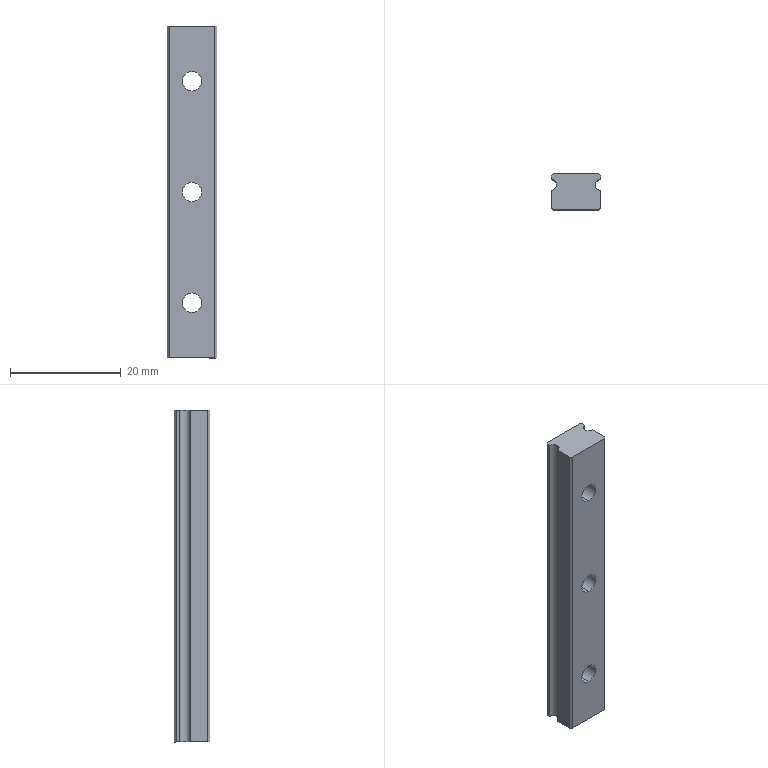Part | SolidWorks | features BaseBody 1, ICE 1 | 1 solid | 30 faces | box 9 x 6.5 x 60 mm | volume 2919 mm3 | cylinder 15 | plane 15 | commonest cylinder face diameters 3.5 x6 6 x6 2 x3
STEP:
#1=CARTESIAN_POINT('',(0.,0.,-55.85));
#2=VERTEX_POINT('',#1);
#3=CARTESIAN_POINT('',(0.,0.,-59.35));
#4=VERTEX_POINT('',#3);
#5=CARTESIAN_POINT('',(0.,0.,-57.6));
#6=DIRECTION('',(0.,-1.,0.));
#7=DIRECTION('',(0.,0.,1.));
#8=AXIS2_PLACEMENT_3D('',#5,#6,#7);
#9=CIRCLE('',#8,1.75);
#10=EDGE_CURVE('',#2,#4,#9,.T.);
#11=ORIENTED_EDGE('',*,*,#10,.T.);
#12=CARTESIAN_POINT('',(0.,3.,-59.35));
#13=VERTEX_POINT('',#12);
#14=CARTESIAN_POINT('',(0.,-94.114,-59.35));
#15=DIRECTION('',(0.,1.,0.));
#16=VECTOR('',#15,1000.);
#17=LINE('',#14,#16);
#18=EDGE_CURVE('',#4,#13,#17,.T.);
#19=ORIENTED_EDGE('',*,*,#18,.T.);
#20=CARTESIAN_POINT('',(0.,3.,-55.85));
#21=VERTEX_POINT('',#20);
#22=CARTESIAN_POINT('',(0.,3.,-57.6));
#23=DIRECTION('',(0.,-1.,0.));
#24=DIRECTION('',(0.,0.,1.));
#25=AXIS2_PLACEMENT_3D('',#22,#23,#24);
#26=CIRCLE('',#25,1.75);
#27=EDGE_CURVE('',#21,#13,#26,.T.);
#28=ORIENTED_EDGE('',*,*,#27,.F.);
#29=CARTESIAN_POINT('',(0.,-94.114,-55.85));
#30=DIRECTION('',(0.,1.,0.));
#31=VECTOR('',#30,1000.);
#32=LINE('',#29,#31);
#33=EDGE_CURVE('',#2,#21,#32,.T.);
#34=ORIENTED_EDGE('',*,*,#33,.F.);
#35=EDGE_LOOP('',(#11,#19,#28,#34));
#36=FACE_OUTER_BOUND('',#35,.T.);
#37=CARTESIAN_POINT('',(0.,-94.114,-57.6));
#38=DIRECTION('',(0.,1.,0.));
#39=DIRECTION('',(0.,0.,1.));
#40=AXIS2_PLACEMENT_3D('',#37,#38,#39);
#41=CYLINDRICAL_SURFACE('',#40,1.75);
#42=ADVANCED_FACE('',(#36),#41,.F.);
#43=CARTESIAN_POINT('',(0.,0.,-75.85));
#44=VERTEX_POINT('',#43);
#45=CARTESIAN_POINT('',(0.,0.,-79.35));
#46=VERTEX_POINT('',#45);
#47=CARTESIAN_POINT('',(0.,0.,-77.6));
#48=DIRECTION('',(0.,-1.,0.));
#49=DIRECTION('',(0.,0.,1.));
#50=AXIS2_PLACEMENT_3D('',#47,#48,#49);
#51=CIRCLE('',#50,1.75);
#52=EDGE_CURVE('',#44,#46,#51,.T.);
#53=ORIENTED_EDGE('',*,*,#52,.T.);
#54=CARTESIAN_POINT('',(0.,3.,-79.35));
#55=VERTEX_POINT('',#54);
#56=CARTESIAN_POINT('',(0.,-94.114,-79.35));
#57=DIRECTION('',(0.,1.,0.));
#58=VECTOR('',#57,1000.);
#59=LINE('',#56,#58);
#60=EDGE_CURVE('',#46,#55,#59,.T.);
#61=ORIENTED_EDGE('',*,*,#60,.T.);
#62=CARTESIAN_POINT('',(0.,3.,-75.85));
#63=VERTEX_POINT('',#62);
#64=CARTESIAN_POINT('',(0.,3.,-77.6));
#65=DIRECTION('',(0.,-1.,0.));
#66=DIRECTION('',(0.,0.,1.));
#67=AXIS2_PLACEMENT_3D('',#64,#65,#66);
#68=CIRCLE('',#67,1.75);
#69=EDGE_CURVE('',#63,#55,#68,.T.);
#70=ORIENTED_EDGE('',*,*,#69,.F.);
#71=CARTESIAN_POINT('',(0.,-94.114,-75.85));
#72=DIRECTION('',(0.,1.,0.));
#73=VECTOR('',#72,1000.);
#74=LINE('',#71,#73);
#75=EDGE_CURVE('',#44,#63,#74,.T.);
#76=ORIENTED_EDGE('',*,*,#75,.F.);
#77=EDGE_LOOP('',(#53,#61,#70,#76));
#78=FACE_OUTER_BOUND('',#77,.T.);
#79=CARTESIAN_POINT('',(0.,-94.114,-77.6));
#80=DIRECTION('',(0.,1.,0.));
#81=DIRECTION('',(0.,0.,1.));
#82=AXIS2_PLACEMENT_3D('',#79,#80,#81);
#83=CYLINDRICAL_SURFACE('',#82,1.75);
#84=ADVANCED_FACE('',(#78),#83,.F.);
#85=CARTESIAN_POINT('',(0.,0.,-95.85));
#86=VERTEX_POINT('',#85);
#87=CARTESIAN_POINT('',(0.,0.,-99.35));
#88=VERTEX_POINT('',#87);
#89=CARTESIAN_POINT('',(0.,0.,-97.6));
#90=DIRECTION('',(0.,-1.,0.));
#91=DIRECTION('',(0.,0.,1.));
#92=AXIS2_PLACEMENT_3D('',#89,#90,#91);
#93=CIRCLE('',#92,1.75);
#94=EDGE_CURVE('',#86,#88,#93,.T.);
#95=ORIENTED_EDGE('',*,*,#94,.T.);
#96=CARTESIAN_POINT('',(0.,3.,-99.35));
#97=VERTEX_POINT('',#96);
#98=CARTESIAN_POINT('',(0.,-94.114,-99.35));
#99=DIRECTION('',(0.,1.,0.));
#100=VECTOR('',#99,1000.);
#101=LINE('',#98,#100);
#102=EDGE_CURVE('',#88,#97,#101,.T.);
#103=ORIENTED_EDGE('',*,*,#102,.T.);
#104=CARTESIAN_POINT('',(0.,3.,-95.85));
#105=VERTEX_POINT('',#104);
#106=CARTESIAN_POINT('',(0.,3.,-97.6));
#107=DIRECTION('',(0.,-1.,0.));
#108=DIRECTION('',(0.,0.,1.));
#109=AXIS2_PLACEMENT_3D('',#106,#107,#108);
#110=CIRCLE('',#109,1.75);
#111=EDGE_CURVE('',#105,#97,#110,.T.);
#112=ORIENTED_EDGE('',*,*,#111,.F.);
#113=CARTESIAN_POINT('',(0.,-94.114,-95.85));
#114=DIRECTION('',(0.,1.,0.));
#115=VECTOR('',#114,1000.);
#116=LINE('',#113,#115);
#117=EDGE_CURVE('',#86,#105,#116,.T.);
#118=ORIENTED_EDGE('',*,*,#117,.F.);
#119=EDGE_LOOP('',(#95,#103,#112,#118));
#120=FACE_OUTER_BOUND('',#119,.T.);
#121=CARTESIAN_POINT('',(0.,-94.114,-97.6));
#122=DIRECTION('',(0.,1.,0.));
#123=DIRECTION('',(0.,0.,1.));
#124=AXIS2_PLACEMENT_3D('',#121,#122,#123);
#125=CYLINDRICAL_SURFACE('',#124,1.75);
#126=ADVANCED_FACE('',(#120),#125,.F.);
#127=CARTESIAN_POINT('',(4.5,5.5,-47.6));
#128=VERTEX_POINT('',#127);
#129=CARTESIAN_POINT('',(3.5,4.5,-47.6));
#130=VERTEX_POINT('',#129);
#131=CARTESIAN_POINT('',(4.5,4.5,-47.6));
#132=DIRECTION('',(0.,0.,1.));
#133=DIRECTION('',(-1.,0.,0.));
#134=AXIS2_PLACEMENT_3D('',#131,#132,#133);
#135=CIRCLE('',#134,1.);
#136=EDGE_CURVE('',#128,#130,#135,.T.);
#137=ORIENTED_EDGE('',*,*,#136,.T.);
#138=CARTESIAN_POINT('',(3.5,4.5,-107.6));
#139=VERTEX_POINT('',#138);
#140=CARTESIAN_POINT('',(3.5,4.5,27.5));
#141=DIRECTION('',(0.,0.,-1.));
#142=VECTOR('',#141,1000.);
#143=LINE('',#140,#142);
#144=EDGE_CURVE('',#130,#139,#143,.T.);
#145=ORIENTED_EDGE('',*,*,#144,.T.);
#146=CARTESIAN_POINT('',(4.5,5.5,-107.6));
#147=VERTEX_POINT('',#146);
#148=CARTESIAN_POINT('',(4.5,4.5,-107.6));
#149=DIRECTION('',(0.,0.,-1.));
#150=DIRECTION('',(-1.,0.,0.));
#151=AXIS2_PLACEMENT_3D('',#148,#149,#150);
#152=CIRCLE('',#151,1.);
#153=EDGE_CURVE('',#139,#147,#152,.T.);
#154=ORIENTED_EDGE('',*,*,#153,.T.);
#155=CARTESIAN_POINT('',(4.5,5.5,27.5));
#156=DIRECTION('',(0.,0.,-1.));
#157=VECTOR('',#156,1000.);
#158=LINE('',#155,#157);
#159=EDGE_CURVE('',#128,#147,#158,.T.);
#160=ORIENTED_EDGE('',*,*,#159,.F.);
#161=EDGE_LOOP('',(#137,#145,#154,#160));
#162=FACE_OUTER_BOUND('',#161,.T.);
#163=CARTESIAN_POINT('',(4.5,4.5,27.5));
#164=DIRECTION('',(0.,0.,-1.));
#165=DIRECTION('',(-1.,0.,0.));
#166=AXIS2_PLACEMENT_3D('',#163,#164,#165);
#167=CYLINDRICAL_SURFACE('',#166,1.);
#168=ADVANCED_FACE('',(#162),#167,.F.);
#169=CARTESIAN_POINT('',(0.,3.,-60.6));
#170=VERTEX_POINT('',#169);
#171=CARTESIAN_POINT('',(0.,3.,-54.6));
#172=VERTEX_POINT('',#171);
#173=CARTESIAN_POINT('',(0.,3.,-57.6));
#174=DIRECTION('',(0.,1.,0.));
#175=DIRECTION('',(0.,0.,1.));
#176=AXIS2_PLACEMENT_3D('',#173,#174,#175);
#177=CIRCLE('',#176,3.);
#178=EDGE_CURVE('',#170,#172,#177,.T.);
#179=ORIENTED_EDGE('',*,*,#178,.F.);
#180=CARTESIAN_POINT('',(0.,6.5,-60.6));
#181=VERTEX_POINT('',#180);
#182=CARTESIAN_POINT('',(0.,4.75,-60.6));
#183=DIRECTION('',(0.,1.,0.));
#184=VECTOR('',#183,1000.);
#185=LINE('',#182,#184);
#186=EDGE_CURVE('',#170,#181,#185,.T.);
#187=ORIENTED_EDGE('',*,*,#186,.T.);
#188=CARTESIAN_POINT('',(0.,6.5,-54.6));
#189=VERTEX_POINT('',#188);
#190=CARTESIAN_POINT('',(0.,6.5,-57.6));
#191=DIRECTION('',(0.,1.,0.));
#192=DIRECTION('',(0.,0.,1.));
#193=AXIS2_PLACEMENT_3D('',#190,#191,#192);
#194=CIRCLE('',#193,3.);
#195=EDGE_CURVE('',#181,#189,#194,.T.);
#196=ORIENTED_EDGE('',*,*,#195,.T.);
#197=CARTESIAN_POINT('',(0.,4.75,-54.6));
#198=DIRECTION('',(0.,1.,0.));
#199=VECTOR('',#198,1000.);
#200=LINE('',#197,#199);
#201=EDGE_CURVE('',#172,#189,#200,.T.);
#202=ORIENTED_EDGE('',*,*,#201,.F.);
#203=EDGE_LOOP('',(#179,#187,#196,#202));
#204=FACE_OUTER_BOUND('',#203,.T.);
#205=CARTESIAN_POINT('',(0.,4.75,-57.6));
#206=DIRECTION('',(0.,1.,0.));
#207=DIRECTION('',(0.,0.,1.));
#208=AXIS2_PLACEMENT_3D('',#205,#206,#207);
#209=CYLINDRICAL_SURFACE('',#208,3.);
#210=ADVANCED_FACE('',(#204),#209,.F.);
#211=CARTESIAN_POINT('',(0.,3.,-80.6));
#212=VERTEX_POINT('',#211);
#213=CARTESIAN_POINT('',(0.,3.,-74.6));
#214=VERTEX_POINT('',#213);
#215=CARTESIAN_POINT('',(0.,3.,-77.6));
#216=DIRECTION('',(0.,1.,0.));
#217=DIRECTION('',(0.,0.,1.));
#218=AXIS2_PLACEMENT_3D('',#215,#216,#217);
#219=CIRCLE('',#218,3.);
#220=EDGE_CURVE('',#212,#214,#219,.T.);
#221=ORIENTED_EDGE('',*,*,#220,.F.);
#222=CARTESIAN_POINT('',(0.,6.5,-80.6));
#223=VERTEX_POINT('',#222);
#224=CARTESIAN_POINT('',(0.,4.75,-80.6));
#225=DIRECTION('',(0.,1.,0.));
#226=VECTOR('',#225,1000.);
#227=LINE('',#224,#226);
#228=EDGE_CURVE('',#212,#223,#227,.T.);
#229=ORIENTED_EDGE('',*,*,#228,.T.);
#230=CARTESIAN_POINT('',(0.,6.5,-74.6));
#231=VERTEX_POINT('',#230);
#232=CARTESIAN_POINT('',(0.,6.5,-77.6));
#233=DIRECTION('',(0.,1.,0.));
#234=DIRECTION('',(0.,0.,1.));
#235=AXIS2_PLACEMENT_3D('',#232,#233,#234);
#236=CIRCLE('',#235,3.);
#237=EDGE_CURVE('',#223,#231,#236,.T.);
#238=ORIENTED_EDGE('',*,*,#237,.T.);
#239=CARTESIAN_POINT('',(0.,4.75,-74.6));
#240=DIRECTION('',(0.,1.,0.));
#241=VECTOR('',#240,1000.);
#242=LINE('',#239,#241);
#243=EDGE_CURVE('',#214,#231,#242,.T.);
#244=ORIENTED_EDGE('',*,*,#243,.F.);
#245=EDGE_LOOP('',(#221,#229,#238,#244));
#246=FACE_OUTER_BOUND('',#245,.T.);
#247=CARTESIAN_POINT('',(0.,4.75,-77.6));
#248=DIRECTION('',(0.,1.,0.));
#249=DIRECTION('',(0.,0.,1.));
#250=AXIS2_PLACEMENT_3D('',#247,#248,#249);
#251=CYLINDRICAL_SURFACE('',#250,3.);
#252=ADVANCED_FACE('',(#246),#251,.F.);
#253=CARTESIAN_POINT('',(0.,3.,-100.6));
#254=VERTEX_POINT('',#253);
#255=CARTESIAN_POINT('',(0.,3.,-94.6));
#256=VERTEX_POINT('',#255);
#257=CARTESIAN_POINT('',(0.,3.,-97.6));
#258=DIRECTION('',(0.,1.,0.));
#259=DIRECTION('',(0.,0.,1.));
#260=AXIS2_PLACEMENT_3D('',#257,#258,#259);
#261=CIRCLE('',#260,3.);
#262=EDGE_CURVE('',#254,#256,#261,.T.);
#263=ORIENTED_EDGE('',*,*,#262,.F.);
#264=CARTESIAN_POINT('',(0.,6.5,-100.6));
#265=VERTEX_POINT('',#264);
#266=CARTESIAN_POINT('',(0.,4.75,-100.6));
#267=DIRECTION('',(0.,1.,0.));
#268=VECTOR('',#267,1000.);
#269=LINE('',#266,#268);
#270=EDGE_CURVE('',#254,#265,#269,.T.);
#271=ORIENTED_EDGE('',*,*,#270,.T.);
#272=CARTESIAN_POINT('',(0.,6.5,-94.6));
#273=VERTEX_POINT('',#272);
#274=CARTESIAN_POINT('',(0.,6.5,-97.6));
#275=DIRECTION('',(0.,1.,0.));
#276=DIRECTION('',(0.,0.,1.));
#277=AXIS2_PLACEMENT_3D('',#274,#275,#276);
#278=CIRCLE('',#277,3.);
#279=EDGE_CURVE('',#265,#273,#278,.T.);
#280=ORIENTED_EDGE('',*,*,#279,.T.);
#281=CARTESIAN_POINT('',(0.,4.75,-94.6));
#282=DIRECTION('',(0.,1.,0.));
#283=VECTOR('',#282,1000.);
#284=LINE('',#281,#283);
#285=EDGE_CURVE('',#256,#273,#284,.T.);
#286=ORIENTED_EDGE('',*,*,#285,.F.);
#287=EDGE_LOOP('',(#263,#271,#280,#286));
#288=FACE_OUTER_BOUND('',#287,.T.);
#289=CARTESIAN_POINT('',(0.,4.75,-97.6));
#290=DIRECTION('',(0.,1.,0.));
#291=DIRECTION('',(0.,0.,1.));
#292=AXIS2_PLACEMENT_3D('',#289,#290,#291);
#293=CYLINDRICAL_SURFACE('',#292,3.);
#294=ADVANCED_FACE('',(#288),#293,.F.);
#295=ORIENTED_EDGE('',*,*,#10,.F.);
#296=CARTESIAN_POINT('',(0.,0.,-57.6));
#297=DIRECTION('',(0.,-1.,0.));
#298=DIRECTION('',(0.,0.,1.));
#299=AXIS2_PLACEMENT_3D('',#296,#297,#298);
#300=CIRCLE('',#299,1.75);
#301=EDGE_CURVE('',#4,#2,#300,.T.);
#302=ORIENTED_EDGE('',*,*,#301,.F.);
#303=EDGE_LOOP('',(#295,#302));
#304=FACE_BOUND('',#303,.T.);
#305=ORIENTED_EDGE('',*,*,#52,.F.);
#306=CARTESIAN_POINT('',(0.,0.,-77.6));
#307=DIRECTION('',(0.,-1.,0.));
#308=DIRECTION('',(0.,0.,1.));
#309=AXIS2_PLACEMENT_3D('',#306,#307,#308);
#310=CIRCLE('',#309,1.75);
#311=EDGE_CURVE('',#46,#44,#310,.T.);
#312=ORIENTED_EDGE('',*,*,#311,.F.);
#313=EDGE_LOOP('',(#305,#312));
#314=FACE_BOUND('',#313,.T.);
#315=ORIENTED_EDGE('',*,*,#94,.F.);
#316=CARTESIAN_POINT('',(0.,0.,-97.6));
#317=DIRECTION('',(0.,-1.,0.));
#318=DIRECTION('',(0.,0.,1.));
#319=AXIS2_PLACEMENT_3D('',#316,#317,#318);
#320=CIRCLE('',#319,1.75);
#321=EDGE_CURVE('',#88,#86,#320,.T.);
#322=ORIENTED_EDGE('',*,*,#321,.F.);
#323=EDGE_LOOP('',(#315,#322));
#324=FACE_BOUND('',#323,.T.);
#325=CARTESIAN_POINT('',(4.1,0.,-47.6));
#326=VERTEX_POINT('',#325);
#327=CARTESIAN_POINT('',(4.1,0.,-107.6));
#328=VERTEX_POINT('',#327);
#329=CARTESIAN_POINT('',(4.1,0.,27.5));
#330=DIRECTION('',(0.,0.,-1.));
#331=VECTOR('',#330,1000.);
#332=LINE('',#329,#331);
#333=EDGE_CURVE('',#326,#328,#332,.T.);
#334=ORIENTED_EDGE('',*,*,#333,.F.);
#335=CARTESIAN_POINT('',(-4.1,0.,-47.6));
#336=VERTEX_POINT('',#335);
#337=CARTESIAN_POINT('',(-4.5,0.,-47.6));
#338=DIRECTION('',(-1.,0.,0.));
#339=VECTOR('',#338,1000.);
#340=LINE('',#337,#339);
#341=EDGE_CURVE('',#326,#336,#340,.T.);
#342=ORIENTED_EDGE('',*,*,#341,.T.);
#343=CARTESIAN_POINT('',(-4.1,0.,-107.6));
#344=VERTEX_POINT('',#343);
#345=CARTESIAN_POINT('',(-4.1,0.,27.5));
#346=DIRECTION('',(0.,0.,1.));
#347=VECTOR('',#346,1000.);
#348=LINE('',#345,#347);
#349=EDGE_CURVE('',#344,#336,#348,.T.);
#350=ORIENTED_EDGE('',*,*,#349,.F.);
#351=CARTESIAN_POINT('',(-4.5,0.,-107.6));
#352=DIRECTION('',(-1.,0.,0.));
#353=VECTOR('',#352,1000.);
#354=LINE('',#351,#353);
#355=EDGE_CURVE('',#328,#344,#354,.T.);
#356=ORIENTED_EDGE('',*,*,#355,.F.);
#357=EDGE_LOOP('',(#334,#342,#350,#356));
#358=FACE_OUTER_BOUND('',#357,.T.);
#359=CARTESIAN_POINT('',(-4.5,0.,27.5));
#360=DIRECTION('',(0.,1.,0.));
#361=DIRECTION('',(0.,0.,1.));
#362=AXIS2_PLACEMENT_3D('',#359,#360,#361);
#363=PLANE('',#362);
#364=ADVANCED_FACE('',(#304,#314,#324,#358),#363,.F.);
#365=ORIENTED_EDGE('',*,*,#18,.F.);
#366=ORIENTED_EDGE('',*,*,#301,.T.);
#367=ORIENTED_EDGE('',*,*,#33,.T.);
#368=CARTESIAN_POINT('',(0.,3.,-57.6));
#369=DIRECTION('',(0.,-1.,0.));
#370=DIRECTION('',(0.,0.,1.));
#371=AXIS2_PLACEMENT_3D('',#368,#369,#370);
#372=CIRCLE('',#371,1.75);
#373=EDGE_CURVE('',#13,#21,#372,.T.);
#374=ORIENTED_EDGE('',*,*,#373,.F.);
#375=EDGE_LOOP('',(#365,#366,#367,#374));
#376=FACE_OUTER_BOUND('',#375,.T.);
#377=CARTESIAN_POINT('',(0.,-94.114,-57.6));
#378=DIRECTION('',(0.,1.,0.));
#379=DIRECTION('',(0.,0.,1.));
#380=AXIS2_PLACEMENT_3D('',#377,#378,#379);
#381=CYLINDRICAL_SURFACE('',#380,1.75);
#382=ADVANCED_FACE('',(#376),#381,.F.);
#383=ORIENTED_EDGE('',*,*,#60,.F.);
#384=ORIENTED_EDGE('',*,*,#311,.T.);
#385=ORIENTED_EDGE('',*,*,#75,.T.);
#386=CARTESIAN_POINT('',(0.,3.,-77.6));
#387=DIRECTION('',(0.,-1.,0.));
#388=DIRECTION('',(0.,0.,1.));
#389=AXIS2_PLACEMENT_3D('',#386,#387,#388);
#390=CIRCLE('',#389,1.75);
#391=EDGE_CURVE('',#55,#63,#390,.T.);
#392=ORIENTED_EDGE('',*,*,#391,.F.);
#393=EDGE_LOOP('',(#383,#384,#385,#392));
#394=FACE_OUTER_BOUND('',#393,.T.);
#395=CARTESIAN_POINT('',(0.,-94.114,-77.6));
#396=DIRECTION('',(0.,1.,0.));
#397=DIRECTION('',(0.,0.,1.));
#398=AXIS2_PLACEMENT_3D('',#395,#396,#397);
#399=CYLINDRICAL_SURFACE('',#398,1.75);
#400=ADVANCED_FACE('',(#394),#399,.F.);
#401=ORIENTED_EDGE('',*,*,#102,.F.);
#402=ORIENTED_EDGE('',*,*,#321,.T.);
#403=ORIENTED_EDGE('',*,*,#117,.T.);
#404=CARTESIAN_POINT('',(0.,3.,-97.6));
#405=DIRECTION('',(0.,-1.,0.));
#406=DIRECTION('',(0.,0.,1.));
#407=AXIS2_PLACEMENT_3D('',#404,#405,#406);
#408=CIRCLE('',#407,1.75);
#409=EDGE_CURVE('',#97,#105,#408,.T.);
#410=ORIENTED_EDGE('',*,*,#409,.F.);
#411=EDGE_LOOP('',(#401,#402,#403,#410));
#412=FACE_OUTER_BOUND('',#411,.T.);
#413=CARTESIAN_POINT('',(0.,-94.114,-97.6));
#414=DIRECTION('',(0.,1.,0.));
#415=DIRECTION('',(0.,0.,1.));
#416=AXIS2_PLACEMENT_3D('',#413,#414,#415);
#417=CYLINDRICAL_SURFACE('',#416,1.75);
#418=ADVANCED_FACE('',(#412),#417,.F.);
#419=ORIENTED_EDGE('',*,*,#349,.T.);
#420=CARTESIAN_POINT('',(-4.5,0.4,-47.6));
#421=VERTEX_POINT('',#420);
#422=CARTESIAN_POINT('',(-4.1,0.,-47.6));
#423=DIRECTION('',(-0.7071,0.7071,0.));
#424=VECTOR('',#423,1000.);
#425=LINE('',#422,#424);
#426=EDGE_CURVE('',#336,#421,#425,.T.);
#427=ORIENTED_EDGE('',*,*,#426,.T.);
#428=CARTESIAN_POINT('',(-4.5,0.4,-107.6));
#429=VERTEX_POINT('',#428);
#430=CARTESIAN_POINT('',(-4.5,0.4,-7.6));
#431=DIRECTION('',(0.,0.,1.));
#432=VECTOR('',#431,1000.);
#433=LINE('',#430,#432);
#434=EDGE_CURVE('',#429,#421,#433,.T.);
#435=ORIENTED_EDGE('',*,*,#434,.F.);
#436=CARTESIAN_POINT('',(-4.1,0.,-107.6));
#437=DIRECTION('',(-0.7071,0.7071,0.));
#438=VECTOR('',#437,1000.);
#439=LINE('',#436,#438);
#440=EDGE_CURVE('',#344,#429,#439,.T.);
#441=ORIENTED_EDGE('',*,*,#440,.F.);
#442=EDGE_LOOP('',(#419,#427,#435,#441));
#443=FACE_OUTER_BOUND('',#442,.T.);
#444=CARTESIAN_POINT('',(-4.1,0.,-7.6));
#445=DIRECTION('',(0.7071,0.7071,0.));
#446=DIRECTION('',(-0.7071,0.7071,0.));
#447=AXIS2_PLACEMENT_3D('',#444,#445,#446);
#448=PLANE('',#447);
#449=ADVANCED_FACE('',(#443),#448,.F.);
#450=CARTESIAN_POINT('',(4.5,6.1,-107.6));
#451=VERTEX_POINT('',#450);
#452=CARTESIAN_POINT('',(4.5,5.5,-107.6));
#453=DIRECTION('',(0.,-1.,0.));
#454=VECTOR('',#453,1000.);
#455=LINE('',#452,#454);
#456=EDGE_CURVE('',#451,#147,#455,.T.);
#457=ORIENTED_EDGE('',*,*,#456,.T.);
#458=ORIENTED_EDGE('',*,*,#153,.F.);
#459=CARTESIAN_POINT('',(4.5,3.5,-107.6));
#460=VERTEX_POINT('',#459);
#461=CARTESIAN_POINT('',(4.5,4.5,-107.6));
#462=DIRECTION('',(0.,0.,-1.));
#463=DIRECTION('',(-1.,0.,0.));
#464=AXIS2_PLACEMENT_3D('',#461,#462,#463);
#465=CIRCLE('',#464,1.);
#466=EDGE_CURVE('',#460,#139,#465,.T.);
#467=ORIENTED_EDGE('',*,*,#466,.F.);
#468=CARTESIAN_POINT('',(4.5,0.4,-107.6));
#469=VERTEX_POINT('',#468);
#470=CARTESIAN_POINT('',(4.5,3.279,-107.6));
#471=DIRECTION('',(0.,1.,0.));
#472=VECTOR('',#471,1000.);
#473=LINE('',#470,#472);
#474=EDGE_CURVE('',#469,#460,#473,.T.);
#475=ORIENTED_EDGE('',*,*,#474,.F.);
#476=CARTESIAN_POINT('',(4.1,0.,-107.6));
#477=DIRECTION('',(0.7071,0.7071,0.));
#478=VECTOR('',#477,1000.);
#479=LINE('',#476,#478);
#480=EDGE_CURVE('',#328,#469,#479,.T.);
#481=ORIENTED_EDGE('',*,*,#480,.F.);
#482=ORIENTED_EDGE('',*,*,#355,.T.);
#483=ORIENTED_EDGE('',*,*,#440,.T.);
#484=CARTESIAN_POINT('',(-4.5,3.5,-107.6));
#485=VERTEX_POINT('',#484);
#486=CARTESIAN_POINT('',(-4.5,3.279,-107.6));
#487=DIRECTION('',(0.,-1.,0.));
#488=VECTOR('',#487,1000.);
#489=LINE('',#486,#488);
#490=EDGE_CURVE('',#485,#429,#489,.T.);
#491=ORIENTED_EDGE('',*,*,#490,.F.);
#492=CARTESIAN_POINT('',(-4.5,5.5,-107.6));
#493=VERTEX_POINT('',#492);
#494=CARTESIAN_POINT('',(-4.5,4.5,-107.6));
#495=DIRECTION('',(0.,0.,-1.));
#496=DIRECTION('',(-1.,0.,0.));
#497=AXIS2_PLACEMENT_3D('',#494,#495,#496);
#498=CIRCLE('',#497,1.);
#499=EDGE_CURVE('',#493,#485,#498,.T.);
#500=ORIENTED_EDGE('',*,*,#499,.F.);
#501=CARTESIAN_POINT('',(-4.5,6.1,-107.6));
#502=VERTEX_POINT('',#501);
#503=CARTESIAN_POINT('',(-4.5,6.5,-107.6));
#504=DIRECTION('',(0.,1.,0.));
#505=VECTOR('',#504,1000.);
#506=LINE('',#503,#505);
#507=EDGE_CURVE('',#493,#502,#506,.T.);
#508=ORIENTED_EDGE('',*,*,#507,.T.);
#509=CARTESIAN_POINT('',(-4.1,6.5,-107.6));
#510=VERTEX_POINT('',#509);
#511=CARTESIAN_POINT('',(-4.5,6.1,-107.6));
#512=DIRECTION('',(0.7071,0.7071,0.));
#513=VECTOR('',#512,1000.);
#514=LINE('',#511,#513);
#515=EDGE_CURVE('',#502,#510,#514,.T.);
#516=ORIENTED_EDGE('',*,*,#515,.T.);
#517=CARTESIAN_POINT('',(4.1,6.5,-107.6));
#518=VERTEX_POINT('',#517);
#519=CARTESIAN_POINT('',(4.5,6.5,-107.6));
#520=DIRECTION('',(-1.,0.,0.));
#521=VECTOR('',#520,1000.);
#522=LINE('',#519,#521);
#523=EDGE_CURVE('',#518,#510,#522,.T.);
#524=ORIENTED_EDGE('',*,*,#523,.F.);
#525=CARTESIAN_POINT('',(4.1,6.5,-107.6));
#526=DIRECTION('',(0.7071,-0.7071,0.));
#527=VECTOR('',#526,1000.);
#528=LINE('',#525,#527);
#529=EDGE_CURVE('',#518,#451,#528,.T.);
#530=ORIENTED_EDGE('',*,*,#529,.T.);
#531=EDGE_LOOP('',(#457,#458,#467,#475,#481,#482,#483,#491,#500,#508,#516,#524,#530));
#532=FACE_OUTER_BOUND('',#531,.T.);
#533=CARTESIAN_POINT('',(0.,3.279,-107.6));
#534=DIRECTION('',(0.,0.,1.));
#535=DIRECTION('',(1.,0.,0.));
#536=AXIS2_PLACEMENT_3D('',#533,#534,#535);
#537=PLANE('',#536);
#538=ADVANCED_FACE('',(#532),#537,.F.);
#539=CARTESIAN_POINT('',(4.5,0.4,-47.6));
#540=VERTEX_POINT('',#539);
#541=CARTESIAN_POINT('',(4.5,0.4,-7.6));
#542=DIRECTION('',(0.,0.,-1.));
#543=VECTOR('',#542,1000.);
#544=LINE('',#541,#543);
#545=EDGE_CURVE('',#540,#469,#544,.T.);
#546=ORIENTED_EDGE('',*,*,#545,.F.);
#547=CARTESIAN_POINT('',(4.5,0.4,-47.6));
#548=DIRECTION('',(-0.7071,-0.7071,0.));
#549=VECTOR('',#548,1000.);
#550=LINE('',#547,#549);
#551=EDGE_CURVE('',#540,#326,#550,.T.);
#552=ORIENTED_EDGE('',*,*,#551,.T.);
#553=ORIENTED_EDGE('',*,*,#333,.T.);
#554=ORIENTED_EDGE('',*,*,#480,.T.);
#555=EDGE_LOOP('',(#546,#552,#553,#554));
#556=FACE_OUTER_BOUND('',#555,.T.);
#557=CARTESIAN_POINT('',(4.5,0.4,-7.6));
#558=DIRECTION('',(-0.7071,0.7071,0.));
#559=DIRECTION('',(-0.7071,-0.7071,0.));
#560=AXIS2_PLACEMENT_3D('',#557,#558,#559);
#561=PLANE('',#560);
#562=ADVANCED_FACE('',(#556),#561,.F.);
#563=ORIENTED_EDGE('',*,*,#27,.T.);
#564=ORIENTED_EDGE('',*,*,#373,.T.);
#565=EDGE_LOOP('',(#563,#564));
#566=FACE_BOUND('',#565,.T.);
#567=CARTESIAN_POINT('',(0.,3.,-57.6));
#568=DIRECTION('',(0.,1.,0.));
#569=DIRECTION('',(0.,0.,1.));
#570=AXIS2_PLACEMENT_3D('',#567,#568,#569);
#571=CIRCLE('',#570,3.);
#572=EDGE_CURVE('',#172,#170,#571,.T.);
#573=ORIENTED_EDGE('',*,*,#572,.T.);
#574=ORIENTED_EDGE('',*,*,#178,.T.);
#575=EDGE_LOOP('',(#573,#574));
#576=FACE_OUTER_BOUND('',#575,.T.);
#577=CARTESIAN_POINT('',(0.,3.,-57.6));
#578=DIRECTION('',(0.,1.,0.));
#579=DIRECTION('',(0.,0.,1.));
#580=AXIS2_PLACEMENT_3D('',#577,#578,#579);
#581=PLANE('',#580);
#582=ADVANCED_FACE('',(#566,#576),#581,.T.);
#583=ORIENTED_EDGE('',*,*,#69,.T.);
#584=ORIENTED_EDGE('',*,*,#391,.T.);
#585=EDGE_LOOP('',(#583,#584));
#586=FACE_BOUND('',#585,.T.);
#587=CARTESIAN_POINT('',(0.,3.,-77.6));
#588=DIRECTION('',(0.,1.,0.));
#589=DIRECTION('',(0.,0.,1.));
#590=AXIS2_PLACEMENT_3D('',#587,#588,#589);
#591=CIRCLE('',#590,3.);
#592=EDGE_CURVE('',#214,#212,#591,.T.);
#593=ORIENTED_EDGE('',*,*,#592,.T.);
#594=ORIENTED_EDGE('',*,*,#220,.T.);
#595=EDGE_LOOP('',(#593,#594));
#596=FACE_OUTER_BOUND('',#595,.T.);
#597=CARTESIAN_POINT('',(0.,3.,-77.6));
#598=DIRECTION('',(0.,1.,0.));
#599=DIRECTION('',(0.,0.,1.));
#600=AXIS2_PLACEMENT_3D('',#597,#598,#599);
#601=PLANE('',#600);
#602=ADVANCED_FACE('',(#586,#596),#601,.T.);
#603=ORIENTED_EDGE('',*,*,#111,.T.);
#604=ORIENTED_EDGE('',*,*,#409,.T.);
#605=EDGE_LOOP('',(#603,#604));
#606=FACE_BOUND('',#605,.T.);
#607=CARTESIAN_POINT('',(0.,3.,-97.6));
#608=DIRECTION('',(0.,1.,0.));
#609=DIRECTION('',(0.,0.,1.));
#610=AXIS2_PLACEMENT_3D('',#607,#608,#609);
#611=CIRCLE('',#610,3.);
#612=EDGE_CURVE('',#256,#254,#611,.T.);
#613=ORIENTED_EDGE('',*,*,#612,.T.);
#614=ORIENTED_EDGE('',*,*,#262,.T.);
#615=EDGE_LOOP('',(#613,#614));
#616=FACE_OUTER_BOUND('',#615,.T.);
#617=CARTESIAN_POINT('',(0.,3.,-97.6));
#618=DIRECTION('',(0.,1.,0.));
#619=DIRECTION('',(0.,0.,1.));
#620=AXIS2_PLACEMENT_3D('',#617,#618,#619);
#621=PLANE('',#620);
#622=ADVANCED_FACE('',(#606,#616),#621,.T.);
#623=ORIENTED_EDGE('',*,*,#434,.T.);
#624=CARTESIAN_POINT('',(-4.5,3.5,-47.6));
#625=VERTEX_POINT('',#624);
#626=CARTESIAN_POINT('',(-4.5,-13.5,-47.6));
#627=DIRECTION('',(0.,1.,0.));
#628=VECTOR('',#627,1000.);
#629=LINE('',#626,#628);
#630=EDGE_CURVE('',#421,#625,#629,.T.);
#631=ORIENTED_EDGE('',*,*,#630,.T.);
#632=CARTESIAN_POINT('',(-4.5,3.5,27.5));
#633=DIRECTION('',(0.,0.,1.));
#634=VECTOR('',#633,1000.);
#635=LINE('',#632,#634);
#636=EDGE_CURVE('',#485,#625,#635,.T.);
#637=ORIENTED_EDGE('',*,*,#636,.F.);
#638=ORIENTED_EDGE('',*,*,#490,.T.);
#639=EDGE_LOOP('',(#623,#631,#637,#638));
#640=FACE_OUTER_BOUND('',#639,.T.);
#641=CARTESIAN_POINT('',(-4.5,3.5,27.5));
#642=DIRECTION('',(1.,0.,0.));
#643=DIRECTION('',(0.,0.,-1.));
#644=AXIS2_PLACEMENT_3D('',#641,#642,#643);
#645=PLANE('',#644);
#646=ADVANCED_FACE('',(#640),#645,.F.);
#647=ORIENTED_EDGE('',*,*,#144,.F.);
#648=CARTESIAN_POINT('',(4.5,3.5,-47.6));
#649=VERTEX_POINT('',#648);
#650=CARTESIAN_POINT('',(4.5,4.5,-47.6));
#651=DIRECTION('',(0.,0.,1.));
#652=DIRECTION('',(-1.,0.,0.));
#653=AXIS2_PLACEMENT_3D('',#650,#651,#652);
#654=CIRCLE('',#653,1.);
#655=EDGE_CURVE('',#130,#649,#654,.T.);
#656=ORIENTED_EDGE('',*,*,#655,.T.);
#657=CARTESIAN_POINT('',(4.5,3.5,27.5));
#658=DIRECTION('',(0.,0.,1.));
#659=VECTOR('',#658,1000.);
#660=LINE('',#657,#659);
#661=EDGE_CURVE('',#460,#649,#660,.T.);
#662=ORIENTED_EDGE('',*,*,#661,.F.);
#663=ORIENTED_EDGE('',*,*,#466,.T.);
#664=EDGE_LOOP('',(#647,#656,#662,#663));
#665=FACE_OUTER_BOUND('',#664,.T.);
#666=CARTESIAN_POINT('',(4.5,4.5,27.5));
#667=DIRECTION('',(0.,0.,-1.));
#668=DIRECTION('',(-1.,0.,0.));
#669=AXIS2_PLACEMENT_3D('',#666,#667,#668);
#670=CYLINDRICAL_SURFACE('',#669,1.);
#671=ADVANCED_FACE('',(#665),#670,.F.);
#672=ORIENTED_EDGE('',*,*,#661,.T.);
#673=CARTESIAN_POINT('',(4.5,-13.5,-47.6));
#674=DIRECTION('',(0.,1.,0.));
#675=VECTOR('',#674,1000.);
#676=LINE('',#673,#675);
#677=EDGE_CURVE('',#540,#649,#676,.T.);
#678=ORIENTED_EDGE('',*,*,#677,.F.);
#679=ORIENTED_EDGE('',*,*,#545,.T.);
#680=ORIENTED_EDGE('',*,*,#474,.T.);
#681=EDGE_LOOP('',(#672,#678,#679,#680));
#682=FACE_OUTER_BOUND('',#681,.T.);
#683=CARTESIAN_POINT('',(4.5,0.,27.5));
#684=DIRECTION('',(-1.,0.,0.));
#685=DIRECTION('',(0.,0.,1.));
#686=AXIS2_PLACEMENT_3D('',#683,#684,#685);
#687=PLANE('',#686);
#688=ADVANCED_FACE('',(#682),#687,.F.);
#689=ORIENTED_EDGE('',*,*,#636,.T.);
#690=CARTESIAN_POINT('',(-4.5,5.5,-47.6));
#691=VERTEX_POINT('',#690);
#692=CARTESIAN_POINT('',(-4.5,4.5,-47.6));
#693=DIRECTION('',(0.,0.,1.));
#694=DIRECTION('',(-1.,0.,0.));
#695=AXIS2_PLACEMENT_3D('',#692,#693,#694);
#696=CIRCLE('',#695,1.);
#697=EDGE_CURVE('',#625,#691,#696,.T.);
#698=ORIENTED_EDGE('',*,*,#697,.T.);
#699=CARTESIAN_POINT('',(-4.5,5.5,27.5));
#700=DIRECTION('',(0.,0.,1.));
#701=VECTOR('',#700,1000.);
#702=LINE('',#699,#701);
#703=EDGE_CURVE('',#493,#691,#702,.T.);
#704=ORIENTED_EDGE('',*,*,#703,.F.);
#705=ORIENTED_EDGE('',*,*,#499,.T.);
#706=EDGE_LOOP('',(#689,#698,#704,#705));
#707=FACE_OUTER_BOUND('',#706,.T.);
#708=CARTESIAN_POINT('',(-4.5,4.5,27.5));
#709=DIRECTION('',(0.,0.,-1.));
#710=DIRECTION('',(-1.,0.,0.));
#711=AXIS2_PLACEMENT_3D('',#708,#709,#710);
#712=CYLINDRICAL_SURFACE('',#711,1.);
#713=ADVANCED_FACE('',(#707),#712,.F.);
#714=CARTESIAN_POINT('',(0.,6.5,-57.6));
#715=DIRECTION('',(0.,1.,0.));
#716=DIRECTION('',(0.,0.,1.));
#717=AXIS2_PLACEMENT_3D('',#714,#715,#716);
#718=CIRCLE('',#717,3.);
#719=EDGE_CURVE('',#189,#181,#718,.T.);
#720=ORIENTED_EDGE('',*,*,#719,.F.);
#721=ORIENTED_EDGE('',*,*,#195,.F.);
#722=EDGE_LOOP('',(#720,#721));
#723=FACE_BOUND('',#722,.T.);
#724=CARTESIAN_POINT('',(0.,6.5,-77.6));
#725=DIRECTION('',(0.,1.,0.));
#726=DIRECTION('',(0.,0.,1.));
#727=AXIS2_PLACEMENT_3D('',#724,#725,#726);
#728=CIRCLE('',#727,3.);
#729=EDGE_CURVE('',#231,#223,#728,.T.);
#730=ORIENTED_EDGE('',*,*,#729,.F.);
#731=ORIENTED_EDGE('',*,*,#237,.F.);
#732=EDGE_LOOP('',(#730,#731));
#733=FACE_BOUND('',#732,.T.);
#734=CARTESIAN_POINT('',(0.,6.5,-97.6));
#735=DIRECTION('',(0.,1.,0.));
#736=DIRECTION('',(0.,0.,1.));
#737=AXIS2_PLACEMENT_3D('',#734,#735,#736);
#738=CIRCLE('',#737,3.);
#739=EDGE_CURVE('',#273,#265,#738,.T.);
#740=ORIENTED_EDGE('',*,*,#739,.F.);
#741=ORIENTED_EDGE('',*,*,#279,.F.);
#742=EDGE_LOOP('',(#740,#741));
#743=FACE_BOUND('',#742,.T.);
#744=CARTESIAN_POINT('',(-4.1,6.5,-47.6));
#745=VERTEX_POINT('',#744);
#746=CARTESIAN_POINT('',(-4.1,6.5,-7.6));
#747=DIRECTION('',(0.,0.,-1.));
#748=VECTOR('',#747,1000.);
#749=LINE('',#746,#748);
#750=EDGE_CURVE('',#745,#510,#749,.T.);
#751=ORIENTED_EDGE('',*,*,#750,.F.);
#752=CARTESIAN_POINT('',(4.1,6.5,-47.6));
#753=VERTEX_POINT('',#752);
#754=CARTESIAN_POINT('',(-4.5,6.5,-47.6));
#755=DIRECTION('',(-1.,0.,0.));
#756=VECTOR('',#755,1000.);
#757=LINE('',#754,#756);
#758=EDGE_CURVE('',#753,#745,#757,.T.);
#759=ORIENTED_EDGE('',*,*,#758,.F.);
#760=CARTESIAN_POINT('',(4.1,6.5,-7.6));
#761=DIRECTION('',(0.,0.,1.));
#762=VECTOR('',#761,1000.);
#763=LINE('',#760,#762);
#764=EDGE_CURVE('',#518,#753,#763,.T.);
#765=ORIENTED_EDGE('',*,*,#764,.F.);
#766=ORIENTED_EDGE('',*,*,#523,.T.);
#767=EDGE_LOOP('',(#751,#759,#765,#766));
#768=FACE_OUTER_BOUND('',#767,.T.);
#769=CARTESIAN_POINT('',(4.5,6.5,27.5));
#770=DIRECTION('',(0.,-1.,0.));
#771=DIRECTION('',(0.,0.,-1.));
#772=AXIS2_PLACEMENT_3D('',#769,#770,#771);
#773=PLANE('',#772);
#774=ADVANCED_FACE('',(#723,#733,#743,#768),#773,.F.);
#775=ORIENTED_EDGE('',*,*,#186,.F.);
#776=ORIENTED_EDGE('',*,*,#572,.F.);
#777=ORIENTED_EDGE('',*,*,#201,.T.);
#778=ORIENTED_EDGE('',*,*,#719,.T.);
#779=EDGE_LOOP('',(#775,#776,#777,#778));
#780=FACE_OUTER_BOUND('',#779,.T.);
#781=CARTESIAN_POINT('',(0.,4.75,-57.6));
#782=DIRECTION('',(0.,1.,0.));
#783=DIRECTION('',(0.,0.,1.));
#784=AXIS2_PLACEMENT_3D('',#781,#782,#783);
#785=CYLINDRICAL_SURFACE('',#784,3.);
#786=ADVANCED_FACE('',(#780),#785,.F.);
#787=ORIENTED_EDGE('',*,*,#228,.F.);
#788=ORIENTED_EDGE('',*,*,#592,.F.);
#789=ORIENTED_EDGE('',*,*,#243,.T.);
#790=ORIENTED_EDGE('',*,*,#729,.T.);
#791=EDGE_LOOP('',(#787,#788,#789,#790));
#792=FACE_OUTER_BOUND('',#791,.T.);
#793=CARTESIAN_POINT('',(0.,4.75,-77.6));
#794=DIRECTION('',(0.,1.,0.));
#795=DIRECTION('',(0.,0.,1.));
#796=AXIS2_PLACEMENT_3D('',#793,#794,#795);
#797=CYLINDRICAL_SURFACE('',#796,3.);
#798=ADVANCED_FACE('',(#792),#797,.F.);
#799=ORIENTED_EDGE('',*,*,#270,.F.);
#800=ORIENTED_EDGE('',*,*,#612,.F.);
#801=ORIENTED_EDGE('',*,*,#285,.T.);
#802=ORIENTED_EDGE('',*,*,#739,.T.);
#803=EDGE_LOOP('',(#799,#800,#801,#802));
#804=FACE_OUTER_BOUND('',#803,.T.);
#805=CARTESIAN_POINT('',(0.,4.75,-97.6));
#806=DIRECTION('',(0.,1.,0.));
#807=DIRECTION('',(0.,0.,1.));
#808=AXIS2_PLACEMENT_3D('',#805,#806,#807);
#809=CYLINDRICAL_SURFACE('',#808,3.);
#810=ADVANCED_FACE('',(#804),#809,.F.);
#811=CARTESIAN_POINT('',(4.5,6.1,-47.6));
#812=VERTEX_POINT('',#811);
#813=CARTESIAN_POINT('',(4.5,6.1,27.5));
#814=DIRECTION('',(0.,0.,-1.));
#815=VECTOR('',#814,1000.);
#816=LINE('',#813,#815);
#817=EDGE_CURVE('',#812,#451,#816,.T.);
#818=ORIENTED_EDGE('',*,*,#817,.F.);
#819=CARTESIAN_POINT('',(4.5,-13.5,-47.6));
#820=DIRECTION('',(0.,1.,0.));
#821=VECTOR('',#820,1000.);
#822=LINE('',#819,#821);
#823=EDGE_CURVE('',#128,#812,#822,.T.);
#824=ORIENTED_EDGE('',*,*,#823,.F.);
#825=ORIENTED_EDGE('',*,*,#159,.T.);
#826=ORIENTED_EDGE('',*,*,#456,.F.);
#827=EDGE_LOOP('',(#818,#824,#825,#826));
#828=FACE_OUTER_BOUND('',#827,.T.);
#829=CARTESIAN_POINT('',(4.5,5.5,27.5));
#830=DIRECTION('',(-1.,0.,0.));
#831=DIRECTION('',(0.,0.,1.));
#832=AXIS2_PLACEMENT_3D('',#829,#830,#831);
#833=PLANE('',#832);
#834=ADVANCED_FACE('',(#828),#833,.F.);
#835=ORIENTED_EDGE('',*,*,#703,.T.);
#836=CARTESIAN_POINT('',(-4.5,6.1,-47.6));
#837=VERTEX_POINT('',#836);
#838=CARTESIAN_POINT('',(-4.5,-13.5,-47.6));
#839=DIRECTION('',(0.,1.,0.));
#840=VECTOR('',#839,1000.);
#841=LINE('',#838,#840);
#842=EDGE_CURVE('',#691,#837,#841,.T.);
#843=ORIENTED_EDGE('',*,*,#842,.T.);
#844=CARTESIAN_POINT('',(-4.5,6.1,27.5));
#845=DIRECTION('',(0.,0.,1.));
#846=VECTOR('',#845,1000.);
#847=LINE('',#844,#846);
#848=EDGE_CURVE('',#502,#837,#847,.T.);
#849=ORIENTED_EDGE('',*,*,#848,.F.);
#850=ORIENTED_EDGE('',*,*,#507,.F.);
#851=EDGE_LOOP('',(#835,#843,#849,#850));
#852=FACE_OUTER_BOUND('',#851,.T.);
#853=CARTESIAN_POINT('',(-4.5,6.5,27.5));
#854=DIRECTION('',(1.,0.,0.));
#855=DIRECTION('',(0.,0.,-1.));
#856=AXIS2_PLACEMENT_3D('',#853,#854,#855);
#857=PLANE('',#856);
#858=ADVANCED_FACE('',(#852),#857,.F.);
#859=ORIENTED_EDGE('',*,*,#764,.T.);
#860=CARTESIAN_POINT('',(4.1,6.5,-47.6));
#861=DIRECTION('',(0.7071,-0.7071,0.));
#862=VECTOR('',#861,1000.);
#863=LINE('',#860,#862);
#864=EDGE_CURVE('',#753,#812,#863,.T.);
#865=ORIENTED_EDGE('',*,*,#864,.T.);
#866=ORIENTED_EDGE('',*,*,#817,.T.);
#867=ORIENTED_EDGE('',*,*,#529,.F.);
#868=EDGE_LOOP('',(#859,#865,#866,#867));
#869=FACE_OUTER_BOUND('',#868,.T.);
#870=CARTESIAN_POINT('',(4.1,6.5,-7.6));
#871=DIRECTION('',(-0.7071,-0.7071,0.));
#872=DIRECTION('',(0.7071,-0.7071,0.));
#873=AXIS2_PLACEMENT_3D('',#870,#871,#872);
#874=PLANE('',#873);
#875=ADVANCED_FACE('',(#869),#874,.F.);
#876=ORIENTED_EDGE('',*,*,#848,.T.);
#877=CARTESIAN_POINT('',(-4.5,6.1,-47.6));
#878=DIRECTION('',(0.7071,0.7071,0.));
#879=VECTOR('',#878,1000.);
#880=LINE('',#877,#879);
#881=EDGE_CURVE('',#837,#745,#880,.T.);
#882=ORIENTED_EDGE('',*,*,#881,.T.);
#883=ORIENTED_EDGE('',*,*,#750,.T.);
#884=ORIENTED_EDGE('',*,*,#515,.F.);
#885=EDGE_LOOP('',(#876,#882,#883,#884));
#886=FACE_OUTER_BOUND('',#885,.T.);
#887=CARTESIAN_POINT('',(-4.5,6.1,-7.6));
#888=DIRECTION('',(0.7071,-0.7071,0.));
#889=DIRECTION('',(0.7071,0.7071,0.));
#890=AXIS2_PLACEMENT_3D('',#887,#888,#889);
#891=PLANE('',#890);
#892=ADVANCED_FACE('',(#886),#891,.F.);
#893=ORIENTED_EDGE('',*,*,#842,.F.);
#894=ORIENTED_EDGE('',*,*,#697,.F.);
#895=ORIENTED_EDGE('',*,*,#630,.F.);
#896=ORIENTED_EDGE('',*,*,#426,.F.);
#897=ORIENTED_EDGE('',*,*,#341,.F.);
#898=ORIENTED_EDGE('',*,*,#551,.F.);
#899=ORIENTED_EDGE('',*,*,#677,.T.);
#900=ORIENTED_EDGE('',*,*,#655,.F.);
#901=ORIENTED_EDGE('',*,*,#136,.F.);
#902=ORIENTED_EDGE('',*,*,#823,.T.);
#903=ORIENTED_EDGE('',*,*,#864,.F.);
#904=ORIENTED_EDGE('',*,*,#758,.T.);
#905=ORIENTED_EDGE('',*,*,#881,.F.);
#906=EDGE_LOOP('',(#893,#894,#895,#896,#897,#898,#899,#900,#901,#902,#903,#904,#905));
#907=FACE_OUTER_BOUND('',#906,.T.);
#908=CARTESIAN_POINT('',(-4.5,-13.5,-47.6));
#909=DIRECTION('',(0.,0.,-1.));
#910=DIRECTION('',(-1.,0.,0.));
#911=AXIS2_PLACEMENT_3D('',#908,#909,#910);
#912=PLANE('',#911);
#913=ADVANCED_FACE('',(#907),#912,.F.);
#914=CLOSED_SHELL('',(#42,#84,#126,#168,#210,#252,#294,#364,#382,#400,#418,#449,#538,#562,#582,#602,#622,#646,#671,#688,#713,#774,#786,#798,#810,#834,#858,#875,#892,#913));
#915=MANIFOLD_SOLID_BREP('',#914);
#916=CARTESIAN_POINT('',(0.,0.,0.));
#917=DIRECTION('',(0.,0.,1.));
#918=DIRECTION('',(1.,0.,0.));
#919=AXIS2_PLACEMENT_3D('',#916,#917,#918);
#920=(LENGTH_UNIT()NAMED_UNIT(*)SI_UNIT(.MILLI.,.METRE.));
#921=UNCERTAINTY_MEASURE_WITH_UNIT(LENGTH_MEASURE(0.00001),#920,'','');
#922=(NAMED_UNIT(*)PLANE_ANGLE_UNIT()SI_UNIT($,.RADIAN.));
#923=(NAMED_UNIT(*)SI_UNIT($,.STERADIAN.)SOLID_ANGLE_UNIT());
#924=(GEOMETRIC_REPRESENTATION_CONTEXT(3)GLOBAL_UNCERTAINTY_ASSIGNED_CONTEXT((#921))GLOBAL_UNIT_ASSIGNED_CONTEXT((#920,#922,#923))REPRESENTATION_CONTEXT('',''));
#925=ADVANCED_BREP_SHAPE_REPRESENTATION('',(#915,#919),#924);